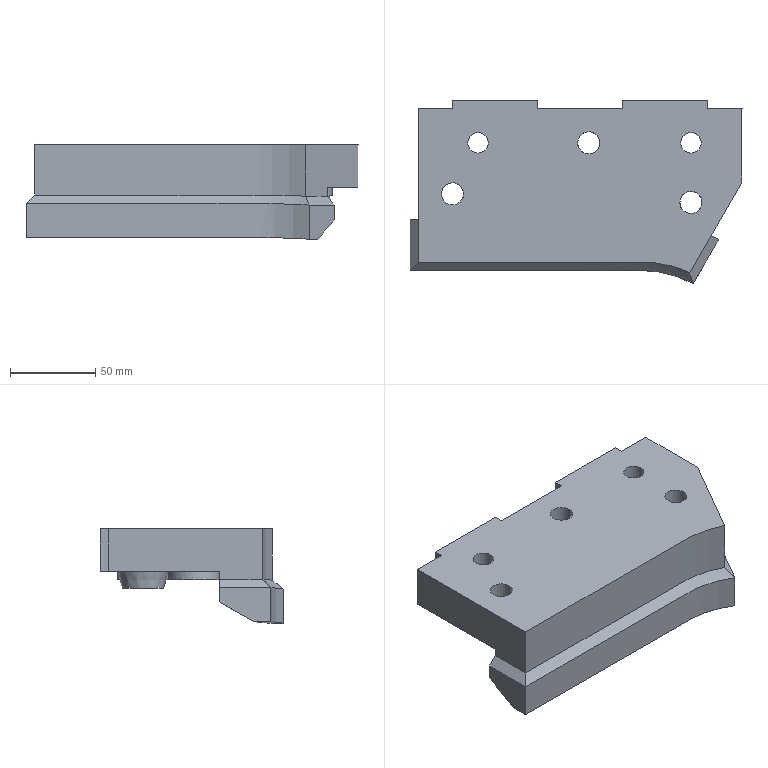Part | NX | features solid 2 | 1 solid | 43 faces | box 195 x 107.704 x 55.432 mm | volume 554737 mm3 | plane 25 | cylinder 10 | spline 6 | cone 2 | commonest cylinder face diameters 13 x5 30 x3 12 x2